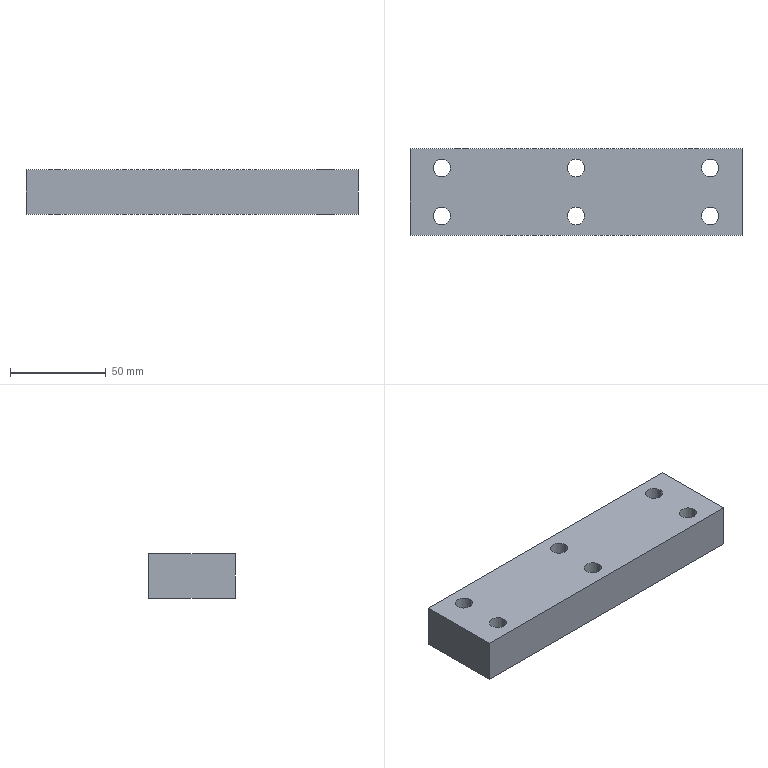Part | STEP file | 44-02-14 Press-fit Locating Plate | 1 solid | 26 faces | box 173 x 45 x 23 mm | volume 168792 mm3 | cylinder 16 | plane 6 | cone 4 | commonest cylinder face diameters 9 x12 6.8 x4